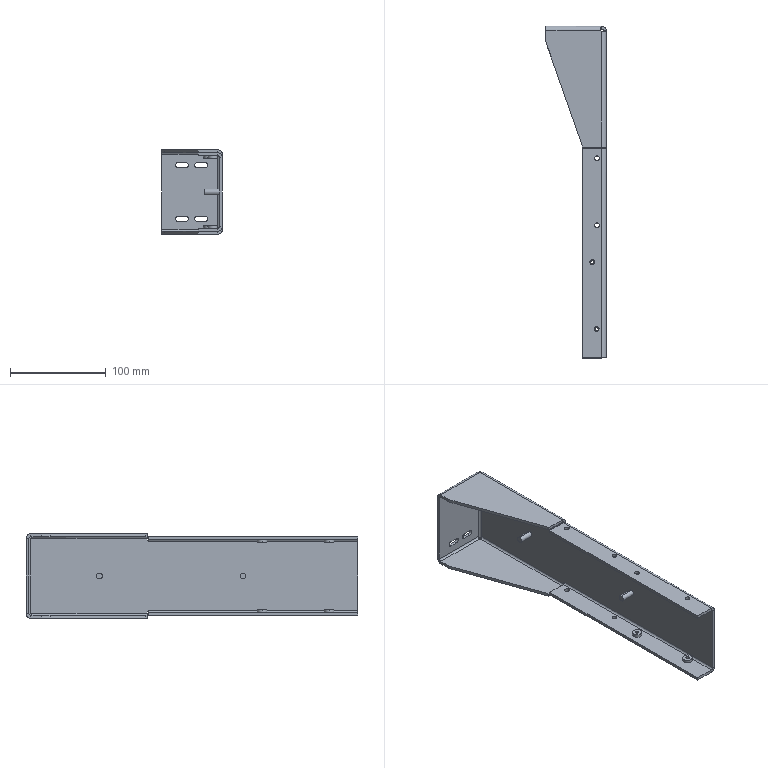Part | SolidWorks | features ICE 7, HoleWzd 5, Chamfer 2, EdgeFlange 2, Cut 1, FlatPattern 1, SMBaseFlange 1, SheetMetal 1 | 1 solid | 136 faces | box 63 x 346.5 x 88 mm | volume 160179 mm3 | plane 70 | cylinder 62 | spline 4 | commonest cylinder face diameters 5 x16 10 x15 5.5 x12 3.3 x8 4 x7 6 x4